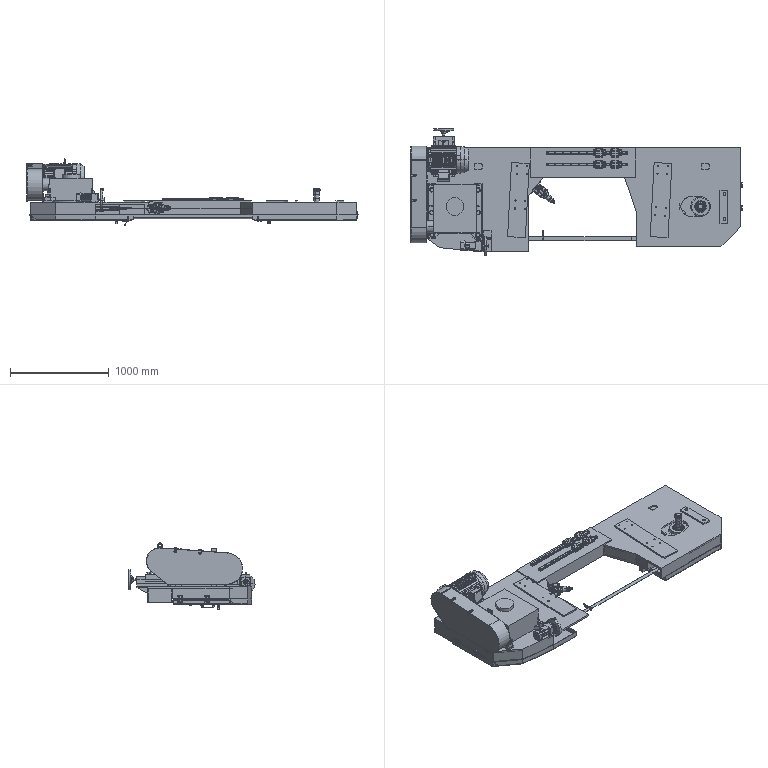Part | SolidWorks | features CompositeCurve 6 | 200 solids | 10371 faces | volume 208271945 mm3 | plane 5103 | cylinder 2771 | cone 1020 | spline 685 | torus 638 | sphere 154 | commonest cylinder face diameters 2.822 x156 12 x139 9 x138 2 x135 2.5 x116 4.2 x100